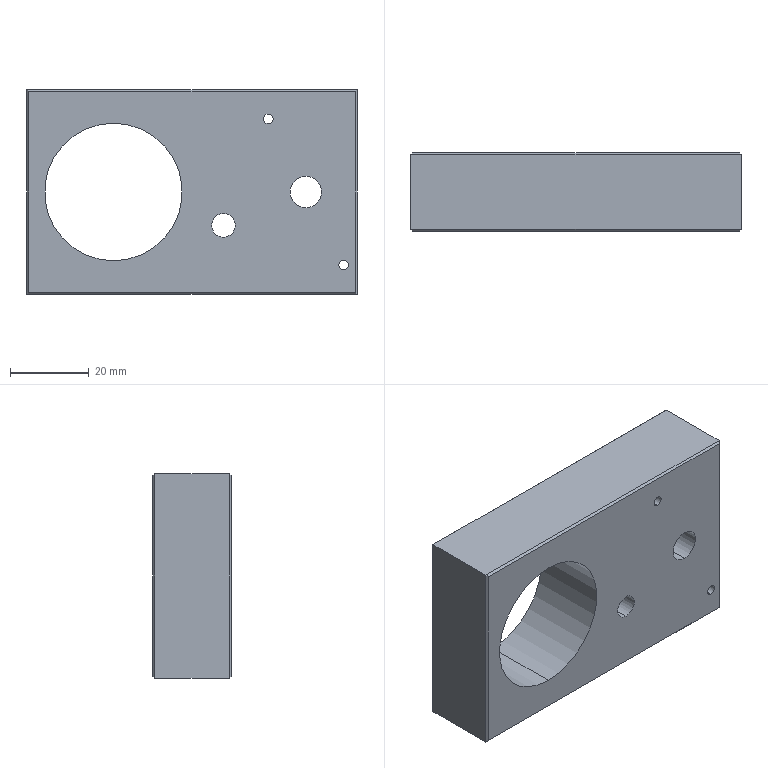Part | SolidWorks | features ICE 5, Chamfer 1, Extrusion 1 | 1 solid | 27 faces | box 84 x 20 x 52 mm | volume 65474 mm3 | plane 15 | cylinder 12 | commonest cylinder face diameters 2.5 x4 6 x2 8 x2 14 x2 35 x2
STEP:
#1=CARTESIAN_POINT('',(29.,12.2,-7.));
#2=VERTEX_POINT('',#1);
#3=CARTESIAN_POINT('',(29.,12.2,7.));
#4=VERTEX_POINT('',#3);
#5=CARTESIAN_POINT('',(29.,12.2,0.));
#6=DIRECTION('',(0.,1.,0.));
#7=DIRECTION('',(0.,0.,1.));
#8=AXIS2_PLACEMENT_3D('',#5,#6,#7);
#9=CIRCLE('',#8,7.);
#10=EDGE_CURVE('',#2,#4,#9,.T.);
#11=ORIENTED_EDGE('',*,*,#10,.F.);
#12=CARTESIAN_POINT('',(29.,20.,-7.));
#13=VERTEX_POINT('',#12);
#14=CARTESIAN_POINT('',(29.,12.2,-7.));
#15=DIRECTION('',(0.,1.,0.));
#16=VECTOR('',#15,1000.);
#17=LINE('',#14,#16);
#18=EDGE_CURVE('',#2,#13,#17,.T.);
#19=ORIENTED_EDGE('',*,*,#18,.T.);
#20=CARTESIAN_POINT('',(29.,20.,7.));
#21=VERTEX_POINT('',#20);
#22=CARTESIAN_POINT('',(29.,20.,0.));
#23=DIRECTION('',(0.,1.,0.));
#24=DIRECTION('',(0.,0.,1.));
#25=AXIS2_PLACEMENT_3D('',#22,#23,#24);
#26=CIRCLE('',#25,7.);
#27=EDGE_CURVE('',#13,#21,#26,.T.);
#28=ORIENTED_EDGE('',*,*,#27,.T.);
#29=CARTESIAN_POINT('',(29.,12.2,7.));
#30=DIRECTION('',(0.,1.,0.));
#31=VECTOR('',#30,1000.);
#32=LINE('',#29,#31);
#33=EDGE_CURVE('',#4,#21,#32,.T.);
#34=ORIENTED_EDGE('',*,*,#33,.F.);
#35=EDGE_LOOP('',(#11,#19,#28,#34));
#36=FACE_OUTER_BOUND('',#35,.T.);
#37=CARTESIAN_POINT('',(29.,12.2,0.));
#38=DIRECTION('',(0.,1.,0.));
#39=DIRECTION('',(0.,0.,1.));
#40=AXIS2_PLACEMENT_3D('',#37,#38,#39);
#41=CYLINDRICAL_SURFACE('',#40,7.);
#42=ADVANCED_FACE('',(#36),#41,.F.);
#43=CARTESIAN_POINT('',(38.6,0.,-19.85));
#44=VERTEX_POINT('',#43);
#45=CARTESIAN_POINT('',(38.6,0.,-17.35));
#46=VERTEX_POINT('',#45);
#47=CARTESIAN_POINT('',(38.6,0.,-18.6));
#48=DIRECTION('',(0.,1.,0.));
#49=DIRECTION('',(0.,0.,1.));
#50=AXIS2_PLACEMENT_3D('',#47,#48,#49);
#51=CIRCLE('',#50,1.25);
#52=EDGE_CURVE('',#44,#46,#51,.T.);
#53=ORIENTED_EDGE('',*,*,#52,.F.);
#54=CARTESIAN_POINT('',(38.6,20.,-19.85));
#55=VERTEX_POINT('',#54);
#56=CARTESIAN_POINT('',(38.6,0.,-19.85));
#57=DIRECTION('',(0.,1.,0.));
#58=VECTOR('',#57,1000.);
#59=LINE('',#56,#58);
#60=EDGE_CURVE('',#44,#55,#59,.T.);
#61=ORIENTED_EDGE('',*,*,#60,.T.);
#62=CARTESIAN_POINT('',(38.6,20.,-17.35));
#63=VERTEX_POINT('',#62);
#64=CARTESIAN_POINT('',(38.6,20.,-18.6));
#65=DIRECTION('',(0.,1.,0.));
#66=DIRECTION('',(0.,0.,1.));
#67=AXIS2_PLACEMENT_3D('',#64,#65,#66);
#68=CIRCLE('',#67,1.25);
#69=EDGE_CURVE('',#55,#63,#68,.T.);
#70=ORIENTED_EDGE('',*,*,#69,.T.);
#71=CARTESIAN_POINT('',(38.6,0.,-17.35));
#72=DIRECTION('',(0.,1.,0.));
#73=VECTOR('',#72,1000.);
#74=LINE('',#71,#73);
#75=EDGE_CURVE('',#46,#63,#74,.T.);
#76=ORIENTED_EDGE('',*,*,#75,.F.);
#77=EDGE_LOOP('',(#53,#61,#70,#76));
#78=FACE_OUTER_BOUND('',#77,.T.);
#79=CARTESIAN_POINT('',(38.6,0.,-18.6));
#80=DIRECTION('',(0.,1.,0.));
#81=DIRECTION('',(0.,0.,1.));
#82=AXIS2_PLACEMENT_3D('',#79,#80,#81);
#83=CYLINDRICAL_SURFACE('',#82,1.25);
#84=ADVANCED_FACE('',(#78),#83,.F.);
#85=CARTESIAN_POINT('',(19.4,0.,17.35));
#86=VERTEX_POINT('',#85);
#87=CARTESIAN_POINT('',(19.4,0.,19.85));
#88=VERTEX_POINT('',#87);
#89=CARTESIAN_POINT('',(19.4,0.,18.6));
#90=DIRECTION('',(0.,1.,0.));
#91=DIRECTION('',(0.,0.,1.));
#92=AXIS2_PLACEMENT_3D('',#89,#90,#91);
#93=CIRCLE('',#92,1.25);
#94=EDGE_CURVE('',#86,#88,#93,.T.);
#95=ORIENTED_EDGE('',*,*,#94,.F.);
#96=CARTESIAN_POINT('',(19.4,20.,17.35));
#97=VERTEX_POINT('',#96);
#98=CARTESIAN_POINT('',(19.4,0.,17.35));
#99=DIRECTION('',(0.,1.,0.));
#100=VECTOR('',#99,1000.);
#101=LINE('',#98,#100);
#102=EDGE_CURVE('',#86,#97,#101,.T.);
#103=ORIENTED_EDGE('',*,*,#102,.T.);
#104=CARTESIAN_POINT('',(19.4,20.,19.85));
#105=VERTEX_POINT('',#104);
#106=CARTESIAN_POINT('',(19.4,20.,18.6));
#107=DIRECTION('',(0.,1.,0.));
#108=DIRECTION('',(0.,0.,1.));
#109=AXIS2_PLACEMENT_3D('',#106,#107,#108);
#110=CIRCLE('',#109,1.25);
#111=EDGE_CURVE('',#97,#105,#110,.T.);
#112=ORIENTED_EDGE('',*,*,#111,.T.);
#113=CARTESIAN_POINT('',(19.4,0.,19.85));
#114=DIRECTION('',(0.,1.,0.));
#115=VECTOR('',#114,1000.);
#116=LINE('',#113,#115);
#117=EDGE_CURVE('',#88,#105,#116,.T.);
#118=ORIENTED_EDGE('',*,*,#117,.F.);
#119=EDGE_LOOP('',(#95,#103,#112,#118));
#120=FACE_OUTER_BOUND('',#119,.T.);
#121=CARTESIAN_POINT('',(19.4,0.,18.6));
#122=DIRECTION('',(0.,1.,0.));
#123=DIRECTION('',(0.,0.,1.));
#124=AXIS2_PLACEMENT_3D('',#121,#122,#123);
#125=CYLINDRICAL_SURFACE('',#124,1.25);
#126=ADVANCED_FACE('',(#120),#125,.F.);
#127=CARTESIAN_POINT('',(8.,0.,-11.5));
#128=VERTEX_POINT('',#127);
#129=CARTESIAN_POINT('',(8.,0.,-5.5));
#130=VERTEX_POINT('',#129);
#131=CARTESIAN_POINT('',(8.,0.,-8.5));
#132=DIRECTION('',(0.,1.,0.));
#133=DIRECTION('',(0.,0.,1.));
#134=AXIS2_PLACEMENT_3D('',#131,#132,#133);
#135=CIRCLE('',#134,3.);
#136=EDGE_CURVE('',#128,#130,#135,.T.);
#137=ORIENTED_EDGE('',*,*,#136,.F.);
#138=CARTESIAN_POINT('',(8.,20.,-11.5));
#139=VERTEX_POINT('',#138);
#140=CARTESIAN_POINT('',(8.,0.,-11.5));
#141=DIRECTION('',(0.,1.,0.));
#142=VECTOR('',#141,1000.);
#143=LINE('',#140,#142);
#144=EDGE_CURVE('',#128,#139,#143,.T.);
#145=ORIENTED_EDGE('',*,*,#144,.T.);
#146=CARTESIAN_POINT('',(8.,20.,-5.5));
#147=VERTEX_POINT('',#146);
#148=CARTESIAN_POINT('',(8.,20.,-8.5));
#149=DIRECTION('',(0.,1.,0.));
#150=DIRECTION('',(0.,0.,1.));
#151=AXIS2_PLACEMENT_3D('',#148,#149,#150);
#152=CIRCLE('',#151,3.);
#153=EDGE_CURVE('',#139,#147,#152,.T.);
#154=ORIENTED_EDGE('',*,*,#153,.T.);
#155=CARTESIAN_POINT('',(8.,0.,-5.5));
#156=DIRECTION('',(0.,1.,0.));
#157=VECTOR('',#156,1000.);
#158=LINE('',#155,#157);
#159=EDGE_CURVE('',#130,#147,#158,.T.);
#160=ORIENTED_EDGE('',*,*,#159,.F.);
#161=EDGE_LOOP('',(#137,#145,#154,#160));
#162=FACE_OUTER_BOUND('',#161,.T.);
#163=CARTESIAN_POINT('',(8.,0.,-8.5));
#164=DIRECTION('',(0.,1.,0.));
#165=DIRECTION('',(0.,0.,1.));
#166=AXIS2_PLACEMENT_3D('',#163,#164,#165);
#167=CYLINDRICAL_SURFACE('',#166,3.);
#168=ADVANCED_FACE('',(#162),#167,.F.);
#169=CARTESIAN_POINT('',(-20.,0.,-17.5));
#170=VERTEX_POINT('',#169);
#171=CARTESIAN_POINT('',(-20.,0.,17.5));
#172=VERTEX_POINT('',#171);
#173=CARTESIAN_POINT('',(-20.,0.,0.));
#174=DIRECTION('',(0.,1.,0.));
#175=DIRECTION('',(0.,0.,1.));
#176=AXIS2_PLACEMENT_3D('',#173,#174,#175);
#177=CIRCLE('',#176,17.5);
#178=EDGE_CURVE('',#170,#172,#177,.T.);
#179=ORIENTED_EDGE('',*,*,#178,.F.);
#180=CARTESIAN_POINT('',(-20.,20.,-17.5));
#181=VERTEX_POINT('',#180);
#182=CARTESIAN_POINT('',(-20.,0.,-17.5));
#183=DIRECTION('',(0.,1.,0.));
#184=VECTOR('',#183,1000.);
#185=LINE('',#182,#184);
#186=EDGE_CURVE('',#170,#181,#185,.T.);
#187=ORIENTED_EDGE('',*,*,#186,.T.);
#188=CARTESIAN_POINT('',(-20.,20.,17.5));
#189=VERTEX_POINT('',#188);
#190=CARTESIAN_POINT('',(-20.,20.,0.));
#191=DIRECTION('',(0.,1.,0.));
#192=DIRECTION('',(0.,0.,1.));
#193=AXIS2_PLACEMENT_3D('',#190,#191,#192);
#194=CIRCLE('',#193,17.5);
#195=EDGE_CURVE('',#181,#189,#194,.T.);
#196=ORIENTED_EDGE('',*,*,#195,.T.);
#197=CARTESIAN_POINT('',(-20.,0.,17.5));
#198=DIRECTION('',(0.,1.,0.));
#199=VECTOR('',#198,1000.);
#200=LINE('',#197,#199);
#201=EDGE_CURVE('',#172,#189,#200,.T.);
#202=ORIENTED_EDGE('',*,*,#201,.F.);
#203=EDGE_LOOP('',(#179,#187,#196,#202));
#204=FACE_OUTER_BOUND('',#203,.T.);
#205=CARTESIAN_POINT('',(-20.,0.,0.));
#206=DIRECTION('',(0.,1.,0.));
#207=DIRECTION('',(0.,0.,1.));
#208=AXIS2_PLACEMENT_3D('',#205,#206,#207);
#209=CYLINDRICAL_SURFACE('',#208,17.5);
#210=ADVANCED_FACE('',(#204),#209,.F.);
#211=CARTESIAN_POINT('',(29.,0.,-4.));
#212=VERTEX_POINT('',#211);
#213=CARTESIAN_POINT('',(29.,0.,4.));
#214=VERTEX_POINT('',#213);
#215=CARTESIAN_POINT('',(29.,0.,0.));
#216=DIRECTION('',(0.,1.,0.));
#217=DIRECTION('',(0.,0.,1.));
#218=AXIS2_PLACEMENT_3D('',#215,#216,#217);
#219=CIRCLE('',#218,4.);
#220=EDGE_CURVE('',#212,#214,#219,.T.);
#221=ORIENTED_EDGE('',*,*,#220,.F.);
#222=CARTESIAN_POINT('',(29.,12.2,-4.));
#223=VERTEX_POINT('',#222);
#224=CARTESIAN_POINT('',(29.,0.,-4.));
#225=DIRECTION('',(0.,1.,0.));
#226=VECTOR('',#225,1000.);
#227=LINE('',#224,#226);
#228=EDGE_CURVE('',#212,#223,#227,.T.);
#229=ORIENTED_EDGE('',*,*,#228,.T.);
#230=CARTESIAN_POINT('',(29.,12.2,4.));
#231=VERTEX_POINT('',#230);
#232=CARTESIAN_POINT('',(29.,12.2,0.));
#233=DIRECTION('',(0.,-1.,0.));
#234=DIRECTION('',(0.,0.,1.));
#235=AXIS2_PLACEMENT_3D('',#232,#233,#234);
#236=CIRCLE('',#235,4.);
#237=EDGE_CURVE('',#231,#223,#236,.T.);
#238=ORIENTED_EDGE('',*,*,#237,.F.);
#239=CARTESIAN_POINT('',(29.,0.,4.));
#240=DIRECTION('',(0.,1.,0.));
#241=VECTOR('',#240,1000.);
#242=LINE('',#239,#241);
#243=EDGE_CURVE('',#214,#231,#242,.T.);
#244=ORIENTED_EDGE('',*,*,#243,.F.);
#245=EDGE_LOOP('',(#221,#229,#238,#244));
#246=FACE_OUTER_BOUND('',#245,.T.);
#247=CARTESIAN_POINT('',(29.,0.,0.));
#248=DIRECTION('',(0.,1.,0.));
#249=DIRECTION('',(0.,0.,1.));
#250=AXIS2_PLACEMENT_3D('',#247,#248,#249);
#251=CYLINDRICAL_SURFACE('',#250,4.);
#252=ADVANCED_FACE('',(#246),#251,.F.);
#253=ORIENTED_EDGE('',*,*,#228,.F.);
#254=CARTESIAN_POINT('',(29.,0.,0.));
#255=DIRECTION('',(0.,1.,0.));
#256=DIRECTION('',(0.,0.,1.));
#257=AXIS2_PLACEMENT_3D('',#254,#255,#256);
#258=CIRCLE('',#257,4.);
#259=EDGE_CURVE('',#214,#212,#258,.T.);
#260=ORIENTED_EDGE('',*,*,#259,.F.);
#261=ORIENTED_EDGE('',*,*,#243,.T.);
#262=CARTESIAN_POINT('',(29.,12.2,0.));
#263=DIRECTION('',(0.,-1.,0.));
#264=DIRECTION('',(0.,0.,1.));
#265=AXIS2_PLACEMENT_3D('',#262,#263,#264);
#266=CIRCLE('',#265,4.);
#267=EDGE_CURVE('',#223,#231,#266,.T.);
#268=ORIENTED_EDGE('',*,*,#267,.F.);
#269=EDGE_LOOP('',(#253,#260,#261,#268));
#270=FACE_OUTER_BOUND('',#269,.T.);
#271=CARTESIAN_POINT('',(29.,0.,0.));
#272=DIRECTION('',(0.,1.,0.));
#273=DIRECTION('',(0.,0.,1.));
#274=AXIS2_PLACEMENT_3D('',#271,#272,#273);
#275=CYLINDRICAL_SURFACE('',#274,4.);
#276=ADVANCED_FACE('',(#270),#275,.F.);
#277=CARTESIAN_POINT('',(42.,19.5,26.));
#278=VERTEX_POINT('',#277);
#279=CARTESIAN_POINT('',(42.,0.5,26.));
#280=VERTEX_POINT('',#279);
#281=CARTESIAN_POINT('',(42.,20.,26.));
#282=DIRECTION('',(0.,-1.,0.));
#283=VECTOR('',#282,1000.);
#284=LINE('',#281,#283);
#285=EDGE_CURVE('',#278,#280,#284,.T.);
#286=ORIENTED_EDGE('',*,*,#285,.T.);
#287=CARTESIAN_POINT('',(42.,0.5,-26.));
#288=VERTEX_POINT('',#287);
#289=CARTESIAN_POINT('',(42.,0.5,-26.));
#290=DIRECTION('',(0.,0.,-1.));
#291=VECTOR('',#290,1000.);
#292=LINE('',#289,#291);
#293=EDGE_CURVE('',#280,#288,#292,.T.);
#294=ORIENTED_EDGE('',*,*,#293,.T.);
#295=CARTESIAN_POINT('',(42.,19.5,-26.));
#296=VERTEX_POINT('',#295);
#297=CARTESIAN_POINT('',(42.,20.,-26.));
#298=DIRECTION('',(0.,-1.,0.));
#299=VECTOR('',#298,1000.);
#300=LINE('',#297,#299);
#301=EDGE_CURVE('',#296,#288,#300,.T.);
#302=ORIENTED_EDGE('',*,*,#301,.F.);
#303=CARTESIAN_POINT('',(42.,19.5,26.));
#304=DIRECTION('',(0.,0.,1.));
#305=VECTOR('',#304,1000.);
#306=LINE('',#303,#305);
#307=EDGE_CURVE('',#296,#278,#306,.T.);
#308=ORIENTED_EDGE('',*,*,#307,.T.);
#309=EDGE_LOOP('',(#286,#294,#302,#308));
#310=FACE_OUTER_BOUND('',#309,.T.);
#311=CARTESIAN_POINT('',(42.,20.,-26.));
#312=DIRECTION('',(-1.,0.,0.));
#313=DIRECTION('',(0.,0.,1.));
#314=AXIS2_PLACEMENT_3D('',#311,#312,#313);
#315=PLANE('',#314);
#316=ADVANCED_FACE('',(#310),#315,.F.);
#317=ORIENTED_EDGE('',*,*,#301,.T.);
#318=CARTESIAN_POINT('',(-42.,0.5,-26.));
#319=VERTEX_POINT('',#318);
#320=CARTESIAN_POINT('',(-42.,0.5,-26.));
#321=DIRECTION('',(-1.,0.,0.));
#322=VECTOR('',#321,1000.);
#323=LINE('',#320,#322);
#324=EDGE_CURVE('',#288,#319,#323,.T.);
#325=ORIENTED_EDGE('',*,*,#324,.T.);
#326=CARTESIAN_POINT('',(-42.,19.5,-26.));
#327=VERTEX_POINT('',#326);
#328=CARTESIAN_POINT('',(-42.,20.,-26.));
#329=DIRECTION('',(0.,-1.,0.));
#330=VECTOR('',#329,1000.);
#331=LINE('',#328,#330);
#332=EDGE_CURVE('',#327,#319,#331,.T.);
#333=ORIENTED_EDGE('',*,*,#332,.F.);
#334=CARTESIAN_POINT('',(42.,19.5,-26.));
#335=DIRECTION('',(1.,0.,0.));
#336=VECTOR('',#335,1000.);
#337=LINE('',#334,#336);
#338=EDGE_CURVE('',#327,#296,#337,.T.);
#339=ORIENTED_EDGE('',*,*,#338,.T.);
#340=EDGE_LOOP('',(#317,#325,#333,#339));
#341=FACE_OUTER_BOUND('',#340,.T.);
#342=CARTESIAN_POINT('',(-42.,20.,-26.));
#343=DIRECTION('',(0.,0.,1.));
#344=DIRECTION('',(1.,0.,0.));
#345=AXIS2_PLACEMENT_3D('',#342,#343,#344);
#346=PLANE('',#345);
#347=ADVANCED_FACE('',(#341),#346,.F.);
#348=ORIENTED_EDGE('',*,*,#332,.T.);
#349=CARTESIAN_POINT('',(-42.,0.5,26.));
#350=VERTEX_POINT('',#349);
#351=CARTESIAN_POINT('',(-42.,0.5,-26.));
#352=DIRECTION('',(0.,0.,1.));
#353=VECTOR('',#352,1000.);
#354=LINE('',#351,#353);
#355=EDGE_CURVE('',#319,#350,#354,.T.);
#356=ORIENTED_EDGE('',*,*,#355,.T.);
#357=CARTESIAN_POINT('',(-42.,19.5,26.));
#358=VERTEX_POINT('',#357);
#359=CARTESIAN_POINT('',(-42.,20.,26.));
#360=DIRECTION('',(0.,-1.,0.));
#361=VECTOR('',#360,1000.);
#362=LINE('',#359,#361);
#363=EDGE_CURVE('',#358,#350,#362,.T.);
#364=ORIENTED_EDGE('',*,*,#363,.F.);
#365=CARTESIAN_POINT('',(-42.,19.5,-26.));
#366=DIRECTION('',(0.,0.,-1.));
#367=VECTOR('',#366,1000.);
#368=LINE('',#365,#367);
#369=EDGE_CURVE('',#358,#327,#368,.T.);
#370=ORIENTED_EDGE('',*,*,#369,.T.);
#371=EDGE_LOOP('',(#348,#356,#364,#370));
#372=FACE_OUTER_BOUND('',#371,.T.);
#373=CARTESIAN_POINT('',(-42.,20.,-26.));
#374=DIRECTION('',(1.,0.,0.));
#375=DIRECTION('',(0.,0.,-1.));
#376=AXIS2_PLACEMENT_3D('',#373,#374,#375);
#377=PLANE('',#376);
#378=ADVANCED_FACE('',(#372),#377,.F.);
#379=ORIENTED_EDGE('',*,*,#363,.T.);
#380=CARTESIAN_POINT('',(-42.,0.5,26.));
#381=DIRECTION('',(1.,0.,0.));
#382=VECTOR('',#381,1000.);
#383=LINE('',#380,#382);
#384=EDGE_CURVE('',#350,#280,#383,.T.);
#385=ORIENTED_EDGE('',*,*,#384,.T.);
#386=ORIENTED_EDGE('',*,*,#285,.F.);
#387=CARTESIAN_POINT('',(-42.,19.5,26.));
#388=DIRECTION('',(-1.,0.,0.));
#389=VECTOR('',#388,1000.);
#390=LINE('',#387,#389);
#391=EDGE_CURVE('',#278,#358,#390,.T.);
#392=ORIENTED_EDGE('',*,*,#391,.T.);
#393=EDGE_LOOP('',(#379,#385,#386,#392));
#394=FACE_OUTER_BOUND('',#393,.T.);
#395=CARTESIAN_POINT('',(-42.,20.,26.));
#396=DIRECTION('',(0.,0.,-1.));
#397=DIRECTION('',(-1.,0.,0.));
#398=AXIS2_PLACEMENT_3D('',#395,#396,#397);
#399=PLANE('',#398);
#400=ADVANCED_FACE('',(#394),#399,.F.);
#401=CARTESIAN_POINT('',(-41.5,20.,25.5));
#402=VERTEX_POINT('',#401);
#403=CARTESIAN_POINT('',(41.5,20.,25.5));
#404=VERTEX_POINT('',#403);
#405=CARTESIAN_POINT('',(42.,20.,25.5));
#406=DIRECTION('',(1.,0.,0.));
#407=VECTOR('',#406,1000.);
#408=LINE('',#405,#407);
#409=EDGE_CURVE('',#402,#404,#408,.T.);
#410=ORIENTED_EDGE('',*,*,#409,.T.);
#411=CARTESIAN_POINT('',(41.5,20.,-25.5));
#412=VERTEX_POINT('',#411);
#413=CARTESIAN_POINT('',(41.5,20.,-26.));
#414=DIRECTION('',(0.,0.,-1.));
#415=VECTOR('',#414,1000.);
#416=LINE('',#413,#415);
#417=EDGE_CURVE('',#404,#412,#416,.T.);
#418=ORIENTED_EDGE('',*,*,#417,.T.);
#419=CARTESIAN_POINT('',(-41.5,20.,-25.5));
#420=VERTEX_POINT('',#419);
#421=CARTESIAN_POINT('',(-42.,20.,-25.5));
#422=DIRECTION('',(-1.,0.,0.));
#423=VECTOR('',#422,1000.);
#424=LINE('',#421,#423);
#425=EDGE_CURVE('',#412,#420,#424,.T.);
#426=ORIENTED_EDGE('',*,*,#425,.T.);
#427=CARTESIAN_POINT('',(-41.5,20.,26.));
#428=DIRECTION('',(0.,0.,1.));
#429=VECTOR('',#428,1000.);
#430=LINE('',#427,#429);
#431=EDGE_CURVE('',#420,#402,#430,.T.);
#432=ORIENTED_EDGE('',*,*,#431,.T.);
#433=EDGE_LOOP('',(#410,#418,#426,#432));
#434=FACE_OUTER_BOUND('',#433,.T.);
#435=CARTESIAN_POINT('',(29.,20.,0.));
#436=DIRECTION('',(0.,1.,0.));
#437=DIRECTION('',(0.,0.,1.));
#438=AXIS2_PLACEMENT_3D('',#435,#436,#437);
#439=CIRCLE('',#438,7.);
#440=EDGE_CURVE('',#21,#13,#439,.T.);
#441=ORIENTED_EDGE('',*,*,#440,.F.);
#442=ORIENTED_EDGE('',*,*,#27,.F.);
#443=EDGE_LOOP('',(#441,#442));
#444=FACE_BOUND('',#443,.T.);
#445=CARTESIAN_POINT('',(38.6,20.,-18.6));
#446=DIRECTION('',(0.,1.,0.));
#447=DIRECTION('',(0.,0.,1.));
#448=AXIS2_PLACEMENT_3D('',#445,#446,#447);
#449=CIRCLE('',#448,1.25);
#450=EDGE_CURVE('',#63,#55,#449,.T.);
#451=ORIENTED_EDGE('',*,*,#450,.F.);
#452=ORIENTED_EDGE('',*,*,#69,.F.);
#453=EDGE_LOOP('',(#451,#452));
#454=FACE_BOUND('',#453,.T.);
#455=CARTESIAN_POINT('',(19.4,20.,18.6));
#456=DIRECTION('',(0.,1.,0.));
#457=DIRECTION('',(0.,0.,1.));
#458=AXIS2_PLACEMENT_3D('',#455,#456,#457);
#459=CIRCLE('',#458,1.25);
#460=EDGE_CURVE('',#105,#97,#459,.T.);
#461=ORIENTED_EDGE('',*,*,#460,.F.);
#462=ORIENTED_EDGE('',*,*,#111,.F.);
#463=EDGE_LOOP('',(#461,#462));
#464=FACE_BOUND('',#463,.T.);
#465=CARTESIAN_POINT('',(8.,20.,-8.5));
#466=DIRECTION('',(0.,1.,0.));
#467=DIRECTION('',(0.,0.,1.));
#468=AXIS2_PLACEMENT_3D('',#465,#466,#467);
#469=CIRCLE('',#468,3.);
#470=EDGE_CURVE('',#147,#139,#469,.T.);
#471=ORIENTED_EDGE('',*,*,#470,.F.);
#472=ORIENTED_EDGE('',*,*,#153,.F.);
#473=EDGE_LOOP('',(#471,#472));
#474=FACE_BOUND('',#473,.T.);
#475=CARTESIAN_POINT('',(-20.,20.,0.));
#476=DIRECTION('',(0.,1.,0.));
#477=DIRECTION('',(0.,0.,1.));
#478=AXIS2_PLACEMENT_3D('',#475,#476,#477);
#479=CIRCLE('',#478,17.5);
#480=EDGE_CURVE('',#189,#181,#479,.T.);
#481=ORIENTED_EDGE('',*,*,#480,.F.);
#482=ORIENTED_EDGE('',*,*,#195,.F.);
#483=EDGE_LOOP('',(#481,#482));
#484=FACE_BOUND('',#483,.T.);
#485=CARTESIAN_POINT('',(0.,20.,0.));
#486=DIRECTION('',(0.,1.,0.));
#487=DIRECTION('',(0.,0.,1.));
#488=AXIS2_PLACEMENT_3D('',#485,#486,#487);
#489=PLANE('',#488);
#490=ADVANCED_FACE('',(#434,#444,#454,#464,#474,#484),#489,.T.);
#491=CARTESIAN_POINT('',(-41.5,0.,25.5));
#492=VERTEX_POINT('',#491);
#493=CARTESIAN_POINT('',(-41.5,0.,-25.5));
#494=VERTEX_POINT('',#493);
#495=CARTESIAN_POINT('',(-41.5,0.,0.));
#496=DIRECTION('',(0.,0.,-1.));
#497=VECTOR('',#496,1000.);
#498=LINE('',#495,#497);
#499=EDGE_CURVE('',#492,#494,#498,.T.);
#500=ORIENTED_EDGE('',*,*,#499,.T.);
#501=CARTESIAN_POINT('',(41.5,0.,-25.5));
#502=VERTEX_POINT('',#501);
#503=CARTESIAN_POINT('',(0.,0.,-25.5));
#504=DIRECTION('',(1.,0.,0.));
#505=VECTOR('',#504,1000.);
#506=LINE('',#503,#505);
#507=EDGE_CURVE('',#494,#502,#506,.T.);
#508=ORIENTED_EDGE('',*,*,#507,.T.);
#509=CARTESIAN_POINT('',(41.5,0.,25.5));
#510=VERTEX_POINT('',#509);
#511=CARTESIAN_POINT('',(41.5,0.,0.));
#512=DIRECTION('',(0.,0.,1.));
#513=VECTOR('',#512,1000.);
#514=LINE('',#511,#513);
#515=EDGE_CURVE('',#502,#510,#514,.T.);
#516=ORIENTED_EDGE('',*,*,#515,.T.);
#517=CARTESIAN_POINT('',(0.,0.,25.5));
#518=DIRECTION('',(-1.,0.,0.));
#519=VECTOR('',#518,1000.);
#520=LINE('',#517,#519);
#521=EDGE_CURVE('',#510,#492,#520,.T.);
#522=ORIENTED_EDGE('',*,*,#521,.T.);
#523=EDGE_LOOP('',(#500,#508,#516,#522));
#524=FACE_OUTER_BOUND('',#523,.T.);
#525=ORIENTED_EDGE('',*,*,#259,.T.);
#526=ORIENTED_EDGE('',*,*,#220,.T.);
#527=EDGE_LOOP('',(#525,#526));
#528=FACE_BOUND('',#527,.T.);
#529=CARTESIAN_POINT('',(38.6,0.,-18.6));
#530=DIRECTION('',(0.,1.,0.));
#531=DIRECTION('',(0.,0.,1.));
#532=AXIS2_PLACEMENT_3D('',#529,#530,#531);
#533=CIRCLE('',#532,1.25);
#534=EDGE_CURVE('',#46,#44,#533,.T.);
#535=ORIENTED_EDGE('',*,*,#534,.T.);
#536=ORIENTED_EDGE('',*,*,#52,.T.);
#537=EDGE_LOOP('',(#535,#536));
#538=FACE_BOUND('',#537,.T.);
#539=CARTESIAN_POINT('',(19.4,0.,18.6));
#540=DIRECTION('',(0.,1.,0.));
#541=DIRECTION('',(0.,0.,1.));
#542=AXIS2_PLACEMENT_3D('',#539,#540,#541);
#543=CIRCLE('',#542,1.25);
#544=EDGE_CURVE('',#88,#86,#543,.T.);
#545=ORIENTED_EDGE('',*,*,#544,.T.);
#546=ORIENTED_EDGE('',*,*,#94,.T.);
#547=EDGE_LOOP('',(#545,#546));
#548=FACE_BOUND('',#547,.T.);
#549=CARTESIAN_POINT('',(8.,0.,-8.5));
#550=DIRECTION('',(0.,1.,0.));
#551=DIRECTION('',(0.,0.,1.));
#552=AXIS2_PLACEMENT_3D('',#549,#550,#551);
#553=CIRCLE('',#552,3.);
#554=EDGE_CURVE('',#130,#128,#553,.T.);
#555=ORIENTED_EDGE('',*,*,#554,.T.);
#556=ORIENTED_EDGE('',*,*,#136,.T.);
#557=EDGE_LOOP('',(#555,#556));
#558=FACE_BOUND('',#557,.T.);
#559=CARTESIAN_POINT('',(-20.,0.,0.));
#560=DIRECTION('',(0.,1.,0.));
#561=DIRECTION('',(0.,0.,1.));
#562=AXIS2_PLACEMENT_3D('',#559,#560,#561);
#563=CIRCLE('',#562,17.5);
#564=EDGE_CURVE('',#172,#170,#563,.T.);
#565=ORIENTED_EDGE('',*,*,#564,.T.);
#566=ORIENTED_EDGE('',*,*,#178,.T.);
#567=EDGE_LOOP('',(#565,#566));
#568=FACE_BOUND('',#567,.T.);
#569=CARTESIAN_POINT('',(0.,0.,0.));
#570=DIRECTION('',(0.,1.,0.));
#571=DIRECTION('',(0.,0.,1.));
#572=AXIS2_PLACEMENT_3D('',#569,#570,#571);
#573=PLANE('',#572);
#574=ADVANCED_FACE('',(#524,#528,#538,#548,#558,#568),#573,.F.);
#575=ORIENTED_EDGE('',*,*,#186,.F.);
#576=ORIENTED_EDGE('',*,*,#564,.F.);
#577=ORIENTED_EDGE('',*,*,#201,.T.);
#578=ORIENTED_EDGE('',*,*,#480,.T.);
#579=EDGE_LOOP('',(#575,#576,#577,#578));
#580=FACE_OUTER_BOUND('',#579,.T.);
#581=CARTESIAN_POINT('',(-20.,0.,0.));
#582=DIRECTION('',(0.,1.,0.));
#583=DIRECTION('',(0.,0.,1.));
#584=AXIS2_PLACEMENT_3D('',#581,#582,#583);
#585=CYLINDRICAL_SURFACE('',#584,17.5);
#586=ADVANCED_FACE('',(#580),#585,.F.);
#587=ORIENTED_EDGE('',*,*,#144,.F.);
#588=ORIENTED_EDGE('',*,*,#554,.F.);
#589=ORIENTED_EDGE('',*,*,#159,.T.);
#590=ORIENTED_EDGE('',*,*,#470,.T.);
#591=EDGE_LOOP('',(#587,#588,#589,#590));
#592=FACE_OUTER_BOUND('',#591,.T.);
#593=CARTESIAN_POINT('',(8.,0.,-8.5));
#594=DIRECTION('',(0.,1.,0.));
#595=DIRECTION('',(0.,0.,1.));
#596=AXIS2_PLACEMENT_3D('',#593,#594,#595);
#597=CYLINDRICAL_SURFACE('',#596,3.);
#598=ADVANCED_FACE('',(#592),#597,.F.);
#599=ORIENTED_EDGE('',*,*,#102,.F.);
#600=ORIENTED_EDGE('',*,*,#544,.F.);
#601=ORIENTED_EDGE('',*,*,#117,.T.);
#602=ORIENTED_EDGE('',*,*,#460,.T.);
#603=EDGE_LOOP('',(#599,#600,#601,#602));
#604=FACE_OUTER_BOUND('',#603,.T.);
#605=CARTESIAN_POINT('',(19.4,0.,18.6));
#606=DIRECTION('',(0.,1.,0.));
#607=DIRECTION('',(0.,0.,1.));
#608=AXIS2_PLACEMENT_3D('',#605,#606,#607);
#609=CYLINDRICAL_SURFACE('',#608,1.25);
#610=ADVANCED_FACE('',(#604),#609,.F.);
#611=ORIENTED_EDGE('',*,*,#60,.F.);
#612=ORIENTED_EDGE('',*,*,#534,.F.);
#613=ORIENTED_EDGE('',*,*,#75,.T.);
#614=ORIENTED_EDGE('',*,*,#450,.T.);
#615=EDGE_LOOP('',(#611,#612,#613,#614));
#616=FACE_OUTER_BOUND('',#615,.T.);
#617=CARTESIAN_POINT('',(38.6,0.,-18.6));
#618=DIRECTION('',(0.,1.,0.));
#619=DIRECTION('',(0.,0.,1.));
#620=AXIS2_PLACEMENT_3D('',#617,#618,#619);
#621=CYLINDRICAL_SURFACE('',#620,1.25);
#622=ADVANCED_FACE('',(#616),#621,.F.);
#623=CARTESIAN_POINT('',(29.,12.2,0.));
#624=DIRECTION('',(0.,1.,0.));
#625=DIRECTION('',(0.,0.,1.));
#626=AXIS2_PLACEMENT_3D('',#623,#624,#625);
#627=CIRCLE('',#626,7.);
#628=EDGE_CURVE('',#4,#2,#627,.T.);
#629=ORIENTED_EDGE('',*,*,#628,.T.);
#630=ORIENTED_EDGE('',*,*,#10,.T.);
#631=EDGE_LOOP('',(#629,#630));
#632=FACE_OUTER_BOUND('',#631,.T.);
#633=ORIENTED_EDGE('',*,*,#237,.T.);
#634=ORIENTED_EDGE('',*,*,#267,.T.);
#635=EDGE_LOOP('',(#633,#634));
#636=FACE_BOUND('',#635,.T.);
#637=CARTESIAN_POINT('',(29.,12.2,0.));
#638=DIRECTION('',(0.,1.,0.));
#639=DIRECTION('',(0.,0.,1.));
#640=AXIS2_PLACEMENT_3D('',#637,#638,#639);
#641=PLANE('',#640);
#642=ADVANCED_FACE('',(#632,#636),#641,.T.);
#643=ORIENTED_EDGE('',*,*,#18,.F.);
#644=ORIENTED_EDGE('',*,*,#628,.F.);
#645=ORIENTED_EDGE('',*,*,#33,.T.);
#646=ORIENTED_EDGE('',*,*,#440,.T.);
#647=EDGE_LOOP('',(#643,#644,#645,#646));
#648=FACE_OUTER_BOUND('',#647,.T.);
#649=CARTESIAN_POINT('',(29.,12.2,0.));
#650=DIRECTION('',(0.,1.,0.));
#651=DIRECTION('',(0.,0.,1.));
#652=AXIS2_PLACEMENT_3D('',#649,#650,#651);
#653=CYLINDRICAL_SURFACE('',#652,7.);
#654=ADVANCED_FACE('',(#648),#653,.F.);
#655=CARTESIAN_POINT('',(-42.,0.5,26.));
#656=DIRECTION('',(-0.5774,0.5774,0.5774));
#657=VECTOR('',#656,1000.);
#658=LINE('',#655,#657);
#659=EDGE_CURVE('',#492,#350,#658,.T.);
#660=ORIENTED_EDGE('',*,*,#659,.F.);
#661=ORIENTED_EDGE('',*,*,#521,.F.);
#662=CARTESIAN_POINT('',(14.,-27.5,-2.));
#663=DIRECTION('',(-0.5774,-0.5774,-0.5774));
#664=VECTOR('',#663,1000.);
#665=LINE('',#662,#664);
#666=EDGE_CURVE('',#280,#510,#665,.T.);
#667=ORIENTED_EDGE('',*,*,#666,.F.);
#668=ORIENTED_EDGE('',*,*,#384,.F.);
#669=EDGE_LOOP('',(#660,#661,#667,#668));
#670=FACE_OUTER_BOUND('',#669,.T.);
#671=CARTESIAN_POINT('',(-42.,0.5,26.));
#672=DIRECTION('',(0.,0.7071,-0.7071));
#673=DIRECTION('',(1.,0.,0.));
#674=AXIS2_PLACEMENT_3D('',#671,#672,#673);
#675=PLANE('',#674);
#676=ADVANCED_FACE('',(#670),#675,.F.);
#677=ORIENTED_EDGE('',*,*,#666,.T.);
#678=ORIENTED_EDGE('',*,*,#515,.F.);
#679=CARTESIAN_POINT('',(42.,0.5,-26.));
#680=DIRECTION('',(-0.5774,-0.5774,0.5774));
#681=VECTOR('',#680,1000.);
#682=LINE('',#679,#681);
#683=EDGE_CURVE('',#288,#502,#682,.T.);
#684=ORIENTED_EDGE('',*,*,#683,.F.);
#685=ORIENTED_EDGE('',*,*,#293,.F.);
#686=EDGE_LOOP('',(#677,#678,#684,#685));
#687=FACE_OUTER_BOUND('',#686,.T.);
#688=CARTESIAN_POINT('',(42.,0.5,-26.));
#689=DIRECTION('',(-0.7071,0.7071,0.));
#690=DIRECTION('',(0.,0.,-1.));
#691=AXIS2_PLACEMENT_3D('',#688,#689,#690);
#692=PLANE('',#691);
#693=ADVANCED_FACE('',(#687),#692,.F.);
#694=ORIENTED_EDGE('',*,*,#659,.T.);
#695=ORIENTED_EDGE('',*,*,#355,.F.);
#696=CARTESIAN_POINT('',(-42.,0.5,-26.));
#697=DIRECTION('',(-0.5774,0.5774,-0.5774));
#698=VECTOR('',#697,1000.);
#699=LINE('',#696,#698);
#700=EDGE_CURVE('',#494,#319,#699,.T.);
#701=ORIENTED_EDGE('',*,*,#700,.F.);
#702=ORIENTED_EDGE('',*,*,#499,.F.);
#703=EDGE_LOOP('',(#694,#695,#701,#702));
#704=FACE_OUTER_BOUND('',#703,.T.);
#705=CARTESIAN_POINT('',(-42.,0.5,-26.));
#706=DIRECTION('',(0.7071,0.7071,0.));
#707=DIRECTION('',(0.,0.,1.));
#708=AXIS2_PLACEMENT_3D('',#705,#706,#707);
#709=PLANE('',#708);
#710=ADVANCED_FACE('',(#704),#709,.F.);
#711=ORIENTED_EDGE('',*,*,#683,.T.);
#712=ORIENTED_EDGE('',*,*,#507,.F.);
#713=ORIENTED_EDGE('',*,*,#700,.T.);
#714=ORIENTED_EDGE('',*,*,#324,.F.);
#715=EDGE_LOOP('',(#711,#712,#713,#714));
#716=FACE_OUTER_BOUND('',#715,.T.);
#717=CARTESIAN_POINT('',(-42.,0.5,-26.));
#718=DIRECTION('',(0.,0.7071,0.7071));
#719=DIRECTION('',(-1.,0.,0.));
#720=AXIS2_PLACEMENT_3D('',#717,#718,#719);
#721=PLANE('',#720);
#722=ADVANCED_FACE('',(#716),#721,.F.);
#723=CARTESIAN_POINT('',(-27.667,33.833,-11.667));
#724=DIRECTION('',(0.5774,0.5774,0.5774));
#725=VECTOR('',#724,1000.);
#726=LINE('',#723,#725);
#727=EDGE_CURVE('',#327,#420,#726,.T.);
#728=ORIENTED_EDGE('',*,*,#727,.F.);
#729=ORIENTED_EDGE('',*,*,#369,.F.);
#730=CARTESIAN_POINT('',(-33.,28.5,17.));
#731=DIRECTION('',(-0.5774,-0.5774,0.5774));
#732=VECTOR('',#731,1000.);
#733=LINE('',#730,#732);
#734=EDGE_CURVE('',#402,#358,#733,.T.);
#735=ORIENTED_EDGE('',*,*,#734,.F.);
#736=ORIENTED_EDGE('',*,*,#431,.F.);
#737=EDGE_LOOP('',(#728,#729,#735,#736));
#738=FACE_OUTER_BOUND('',#737,.T.);
#739=CARTESIAN_POINT('',(-41.5,20.,0.));
#740=DIRECTION('',(-0.7071,0.7071,0.));
#741=DIRECTION('',(0.,0.,-1.));
#742=AXIS2_PLACEMENT_3D('',#739,#740,#741);
#743=PLANE('',#742);
#744=ADVANCED_FACE('',(#738),#743,.T.);
#745=ORIENTED_EDGE('',*,*,#734,.T.);
#746=ORIENTED_EDGE('',*,*,#391,.F.);
#747=CARTESIAN_POINT('',(27.667,33.833,11.667));
#748=DIRECTION('',(0.5774,-0.5774,0.5774));
#749=VECTOR('',#748,1000.);
#750=LINE('',#747,#749);
#751=EDGE_CURVE('',#404,#278,#750,.T.);
#752=ORIENTED_EDGE('',*,*,#751,.F.);
#753=ORIENTED_EDGE('',*,*,#409,.F.);
#754=EDGE_LOOP('',(#745,#746,#752,#753));
#755=FACE_OUTER_BOUND('',#754,.T.);
#756=CARTESIAN_POINT('',(0.,20.,25.5));
#757=DIRECTION('',(0.,0.7071,0.7071));
#758=DIRECTION('',(-1.,0.,0.));
#759=AXIS2_PLACEMENT_3D('',#756,#757,#758);
#760=PLANE('',#759);
#761=ADVANCED_FACE('',(#755),#760,.T.);
#762=ORIENTED_EDGE('',*,*,#727,.T.);
#763=ORIENTED_EDGE('',*,*,#425,.F.);
#764=CARTESIAN_POINT('',(27.667,33.833,-11.667));
#765=DIRECTION('',(-0.5774,0.5774,0.5774));
#766=VECTOR('',#765,1000.);
#767=LINE('',#764,#766);
#768=EDGE_CURVE('',#296,#412,#767,.T.);
#769=ORIENTED_EDGE('',*,*,#768,.F.);
#770=ORIENTED_EDGE('',*,*,#338,.F.);
#771=EDGE_LOOP('',(#762,#763,#769,#770));
#772=FACE_OUTER_BOUND('',#771,.T.);
#773=CARTESIAN_POINT('',(0.,20.,-25.5));
#774=DIRECTION('',(0.,0.7071,-0.7071));
#775=DIRECTION('',(1.,0.,0.));
#776=AXIS2_PLACEMENT_3D('',#773,#774,#775);
#777=PLANE('',#776);
#778=ADVANCED_FACE('',(#772),#777,.T.);
#779=ORIENTED_EDGE('',*,*,#751,.T.);
#780=ORIENTED_EDGE('',*,*,#307,.F.);
#781=ORIENTED_EDGE('',*,*,#768,.T.);
#782=ORIENTED_EDGE('',*,*,#417,.F.);
#783=EDGE_LOOP('',(#779,#780,#781,#782));
#784=FACE_OUTER_BOUND('',#783,.T.);
#785=CARTESIAN_POINT('',(41.5,20.,0.));
#786=DIRECTION('',(0.7071,0.7071,0.));
#787=DIRECTION('',(0.,0.,1.));
#788=AXIS2_PLACEMENT_3D('',#785,#786,#787);
#789=PLANE('',#788);
#790=ADVANCED_FACE('',(#784),#789,.T.);
#791=CLOSED_SHELL('',(#42,#84,#126,#168,#210,#252,#276,#316,#347,#378,#400,#490,#574,#586,#598,#610,#622,#642,#654,#676,#693,#710,#722,#744,#761,#778,#790));
#792=MANIFOLD_SOLID_BREP('',#791);
#793=CARTESIAN_POINT('',(0.,0.,0.));
#794=DIRECTION('',(0.,0.,1.));
#795=DIRECTION('',(1.,0.,0.));
#796=AXIS2_PLACEMENT_3D('',#793,#794,#795);
#797=(LENGTH_UNIT()NAMED_UNIT(*)SI_UNIT(.MILLI.,.METRE.));
#798=UNCERTAINTY_MEASURE_WITH_UNIT(LENGTH_MEASURE(0.00001),#797,'','');
#799=(NAMED_UNIT(*)PLANE_ANGLE_UNIT()SI_UNIT($,.RADIAN.));
#800=(NAMED_UNIT(*)SI_UNIT($,.STERADIAN.)SOLID_ANGLE_UNIT());
#801=(GEOMETRIC_REPRESENTATION_CONTEXT(3)GLOBAL_UNCERTAINTY_ASSIGNED_CONTEXT((#798))GLOBAL_UNIT_ASSIGNED_CONTEXT((#797,#799,#800))REPRESENTATION_CONTEXT('',''));
#802=ADVANCED_BREP_SHAPE_REPRESENTATION('',(#792,#796),#801);